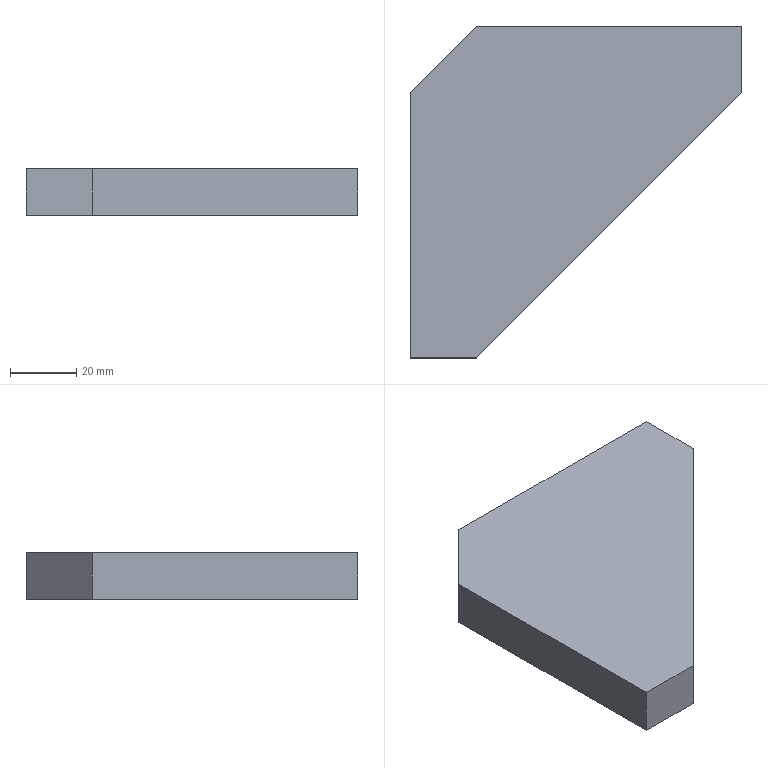Part | SolidWorks | features Extrusion 1 | 1 solid | 8 faces | box 100 x 100 x 14 mm | volume 92400 mm3 | plane 8
STEP:
#1=CARTESIAN_POINT('',(0.,80.,0.));
#2=VERTEX_POINT('',#1);
#3=CARTESIAN_POINT('',(0.,0.,0.));
#4=VERTEX_POINT('',#3);
#5=CARTESIAN_POINT('',(0.,80.,0.));
#6=DIRECTION('',(0.,-1.,0.));
#7=VECTOR('',#6,1000.);
#8=LINE('',#5,#7);
#9=EDGE_CURVE('',#2,#4,#8,.T.);
#10=ORIENTED_EDGE('',*,*,#9,.T.);
#11=CARTESIAN_POINT('',(0.,0.,14.));
#12=VERTEX_POINT('',#11);
#13=CARTESIAN_POINT('',(0.,0.,14.));
#14=DIRECTION('',(0.,0.,-1.));
#15=VECTOR('',#14,1000.);
#16=LINE('',#13,#15);
#17=EDGE_CURVE('',#12,#4,#16,.T.);
#18=ORIENTED_EDGE('',*,*,#17,.F.);
#19=CARTESIAN_POINT('',(0.,80.,14.));
#20=VERTEX_POINT('',#19);
#21=CARTESIAN_POINT('',(0.,80.,14.));
#22=DIRECTION('',(0.,-1.,0.));
#23=VECTOR('',#22,1000.);
#24=LINE('',#21,#23);
#25=EDGE_CURVE('',#20,#12,#24,.T.);
#26=ORIENTED_EDGE('',*,*,#25,.F.);
#27=CARTESIAN_POINT('',(0.,80.,14.));
#28=DIRECTION('',(0.,0.,-1.));
#29=VECTOR('',#28,1000.);
#30=LINE('',#27,#29);
#31=EDGE_CURVE('',#20,#2,#30,.T.);
#32=ORIENTED_EDGE('',*,*,#31,.T.);
#33=EDGE_LOOP('',(#10,#18,#26,#32));
#34=FACE_OUTER_BOUND('',#33,.T.);
#35=CARTESIAN_POINT('',(0.,80.,14.));
#36=DIRECTION('',(1.,0.,0.));
#37=DIRECTION('',(0.,1.,0.));
#38=AXIS2_PLACEMENT_3D('',#35,#36,#37);
#39=PLANE('',#38);
#40=ADVANCED_FACE('',(#34),#39,.F.);
#41=CARTESIAN_POINT('',(20.,0.,0.));
#42=VERTEX_POINT('',#41);
#43=CARTESIAN_POINT('',(0.,0.,0.));
#44=DIRECTION('',(1.,0.,0.));
#45=VECTOR('',#44,1000.);
#46=LINE('',#43,#45);
#47=EDGE_CURVE('',#4,#42,#46,.T.);
#48=ORIENTED_EDGE('',*,*,#47,.T.);
#49=CARTESIAN_POINT('',(20.,0.,14.));
#50=VERTEX_POINT('',#49);
#51=CARTESIAN_POINT('',(20.,0.,14.));
#52=DIRECTION('',(0.,0.,-1.));
#53=VECTOR('',#52,1000.);
#54=LINE('',#51,#53);
#55=EDGE_CURVE('',#50,#42,#54,.T.);
#56=ORIENTED_EDGE('',*,*,#55,.F.);
#57=CARTESIAN_POINT('',(0.,0.,14.));
#58=DIRECTION('',(1.,0.,0.));
#59=VECTOR('',#58,1000.);
#60=LINE('',#57,#59);
#61=EDGE_CURVE('',#12,#50,#60,.T.);
#62=ORIENTED_EDGE('',*,*,#61,.F.);
#63=ORIENTED_EDGE('',*,*,#17,.T.);
#64=EDGE_LOOP('',(#48,#56,#62,#63));
#65=FACE_OUTER_BOUND('',#64,.T.);
#66=CARTESIAN_POINT('',(0.,0.,14.));
#67=DIRECTION('',(0.,1.,0.));
#68=DIRECTION('',(0.,0.,1.));
#69=AXIS2_PLACEMENT_3D('',#66,#67,#68);
#70=PLANE('',#69);
#71=ADVANCED_FACE('',(#65),#70,.F.);
#72=CARTESIAN_POINT('',(100.,80.,0.));
#73=VERTEX_POINT('',#72);
#74=CARTESIAN_POINT('',(20.,0.,0.));
#75=DIRECTION('',(0.7071,0.7071,0.));
#76=VECTOR('',#75,1000.);
#77=LINE('',#74,#76);
#78=EDGE_CURVE('',#42,#73,#77,.T.);
#79=ORIENTED_EDGE('',*,*,#78,.T.);
#80=CARTESIAN_POINT('',(100.,80.,14.));
#81=VERTEX_POINT('',#80);
#82=CARTESIAN_POINT('',(100.,80.,14.));
#83=DIRECTION('',(0.,0.,-1.));
#84=VECTOR('',#83,1000.);
#85=LINE('',#82,#84);
#86=EDGE_CURVE('',#81,#73,#85,.T.);
#87=ORIENTED_EDGE('',*,*,#86,.F.);
#88=CARTESIAN_POINT('',(20.,0.,14.));
#89=DIRECTION('',(0.7071,0.7071,0.));
#90=VECTOR('',#89,1000.);
#91=LINE('',#88,#90);
#92=EDGE_CURVE('',#50,#81,#91,.T.);
#93=ORIENTED_EDGE('',*,*,#92,.F.);
#94=ORIENTED_EDGE('',*,*,#55,.T.);
#95=EDGE_LOOP('',(#79,#87,#93,#94));
#96=FACE_OUTER_BOUND('',#95,.T.);
#97=CARTESIAN_POINT('',(20.,0.,14.));
#98=DIRECTION('',(-0.7071,0.7071,0.));
#99=DIRECTION('',(-0.7071,-0.7071,0.));
#100=AXIS2_PLACEMENT_3D('',#97,#98,#99);
#101=PLANE('',#100);
#102=ADVANCED_FACE('',(#96),#101,.F.);
#103=CARTESIAN_POINT('',(100.,100.,0.));
#104=VERTEX_POINT('',#103);
#105=CARTESIAN_POINT('',(100.,80.,0.));
#106=DIRECTION('',(0.,1.,0.));
#107=VECTOR('',#106,1000.);
#108=LINE('',#105,#107);
#109=EDGE_CURVE('',#73,#104,#108,.T.);
#110=ORIENTED_EDGE('',*,*,#109,.T.);
#111=CARTESIAN_POINT('',(100.,100.,14.));
#112=VERTEX_POINT('',#111);
#113=CARTESIAN_POINT('',(100.,100.,14.));
#114=DIRECTION('',(0.,0.,-1.));
#115=VECTOR('',#114,1000.);
#116=LINE('',#113,#115);
#117=EDGE_CURVE('',#112,#104,#116,.T.);
#118=ORIENTED_EDGE('',*,*,#117,.F.);
#119=CARTESIAN_POINT('',(100.,80.,14.));
#120=DIRECTION('',(0.,1.,0.));
#121=VECTOR('',#120,1000.);
#122=LINE('',#119,#121);
#123=EDGE_CURVE('',#81,#112,#122,.T.);
#124=ORIENTED_EDGE('',*,*,#123,.F.);
#125=ORIENTED_EDGE('',*,*,#86,.T.);
#126=EDGE_LOOP('',(#110,#118,#124,#125));
#127=FACE_OUTER_BOUND('',#126,.T.);
#128=CARTESIAN_POINT('',(100.,80.,14.));
#129=DIRECTION('',(-1.,0.,0.));
#130=DIRECTION('',(0.,0.,1.));
#131=AXIS2_PLACEMENT_3D('',#128,#129,#130);
#132=PLANE('',#131);
#133=ADVANCED_FACE('',(#127),#132,.F.);
#134=CARTESIAN_POINT('',(20.,100.,0.));
#135=VERTEX_POINT('',#134);
#136=CARTESIAN_POINT('',(100.,100.,0.));
#137=DIRECTION('',(-1.,0.,0.));
#138=VECTOR('',#137,1000.);
#139=LINE('',#136,#138);
#140=EDGE_CURVE('',#104,#135,#139,.T.);
#141=ORIENTED_EDGE('',*,*,#140,.T.);
#142=CARTESIAN_POINT('',(20.,100.,14.));
#143=VERTEX_POINT('',#142);
#144=CARTESIAN_POINT('',(20.,100.,14.));
#145=DIRECTION('',(0.,0.,-1.));
#146=VECTOR('',#145,1000.);
#147=LINE('',#144,#146);
#148=EDGE_CURVE('',#143,#135,#147,.T.);
#149=ORIENTED_EDGE('',*,*,#148,.F.);
#150=CARTESIAN_POINT('',(100.,100.,14.));
#151=DIRECTION('',(-1.,0.,0.));
#152=VECTOR('',#151,1000.);
#153=LINE('',#150,#152);
#154=EDGE_CURVE('',#112,#143,#153,.T.);
#155=ORIENTED_EDGE('',*,*,#154,.F.);
#156=ORIENTED_EDGE('',*,*,#117,.T.);
#157=EDGE_LOOP('',(#141,#149,#155,#156));
#158=FACE_OUTER_BOUND('',#157,.T.);
#159=CARTESIAN_POINT('',(100.,100.,14.));
#160=DIRECTION('',(0.,-1.,0.));
#161=DIRECTION('',(1.,0.,0.));
#162=AXIS2_PLACEMENT_3D('',#159,#160,#161);
#163=PLANE('',#162);
#164=ADVANCED_FACE('',(#158),#163,.F.);
#165=CARTESIAN_POINT('',(20.,100.,0.));
#166=DIRECTION('',(-0.7071,-0.7071,0.));
#167=VECTOR('',#166,1000.);
#168=LINE('',#165,#167);
#169=EDGE_CURVE('',#135,#2,#168,.T.);
#170=ORIENTED_EDGE('',*,*,#169,.T.);
#171=ORIENTED_EDGE('',*,*,#31,.F.);
#172=CARTESIAN_POINT('',(20.,100.,14.));
#173=DIRECTION('',(-0.7071,-0.7071,0.));
#174=VECTOR('',#173,1000.);
#175=LINE('',#172,#174);
#176=EDGE_CURVE('',#143,#20,#175,.T.);
#177=ORIENTED_EDGE('',*,*,#176,.F.);
#178=ORIENTED_EDGE('',*,*,#148,.T.);
#179=EDGE_LOOP('',(#170,#171,#177,#178));
#180=FACE_OUTER_BOUND('',#179,.T.);
#181=CARTESIAN_POINT('',(20.,100.,14.));
#182=DIRECTION('',(0.7071,-0.7071,0.));
#183=DIRECTION('',(0.7071,0.7071,0.));
#184=AXIS2_PLACEMENT_3D('',#181,#182,#183);
#185=PLANE('',#184);
#186=ADVANCED_FACE('',(#180),#185,.F.);
#187=ORIENTED_EDGE('',*,*,#25,.T.);
#188=ORIENTED_EDGE('',*,*,#61,.T.);
#189=ORIENTED_EDGE('',*,*,#92,.T.);
#190=ORIENTED_EDGE('',*,*,#123,.T.);
#191=ORIENTED_EDGE('',*,*,#154,.T.);
#192=ORIENTED_EDGE('',*,*,#176,.T.);
#193=EDGE_LOOP('',(#187,#188,#189,#190,#191,#192));
#194=FACE_OUTER_BOUND('',#193,.T.);
#195=CARTESIAN_POINT('',(0.,0.,14.));
#196=DIRECTION('',(0.,0.,1.));
#197=DIRECTION('',(1.,0.,0.));
#198=AXIS2_PLACEMENT_3D('',#195,#196,#197);
#199=PLANE('',#198);
#200=ADVANCED_FACE('',(#194),#199,.T.);
#201=ORIENTED_EDGE('',*,*,#9,.F.);
#202=ORIENTED_EDGE('',*,*,#169,.F.);
#203=ORIENTED_EDGE('',*,*,#140,.F.);
#204=ORIENTED_EDGE('',*,*,#109,.F.);
#205=ORIENTED_EDGE('',*,*,#78,.F.);
#206=ORIENTED_EDGE('',*,*,#47,.F.);
#207=EDGE_LOOP('',(#201,#202,#203,#204,#205,#206));
#208=FACE_OUTER_BOUND('',#207,.T.);
#209=CARTESIAN_POINT('',(0.,0.,0.));
#210=DIRECTION('',(0.,0.,1.));
#211=DIRECTION('',(1.,0.,0.));
#212=AXIS2_PLACEMENT_3D('',#209,#210,#211);
#213=PLANE('',#212);
#214=ADVANCED_FACE('',(#208),#213,.F.);
#215=CLOSED_SHELL('',(#40,#71,#102,#133,#164,#186,#200,#214));
#216=MANIFOLD_SOLID_BREP('',#215);
#217=CARTESIAN_POINT('',(0.,0.,0.));
#218=DIRECTION('',(0.,0.,1.));
#219=DIRECTION('',(1.,0.,0.));
#220=AXIS2_PLACEMENT_3D('',#217,#218,#219);
#221=(LENGTH_UNIT()NAMED_UNIT(*)SI_UNIT(.MILLI.,.METRE.));
#222=UNCERTAINTY_MEASURE_WITH_UNIT(LENGTH_MEASURE(0.00001),#221,'','');
#223=(NAMED_UNIT(*)PLANE_ANGLE_UNIT()SI_UNIT($,.RADIAN.));
#224=(NAMED_UNIT(*)SI_UNIT($,.STERADIAN.)SOLID_ANGLE_UNIT());
#225=(GEOMETRIC_REPRESENTATION_CONTEXT(3)GLOBAL_UNCERTAINTY_ASSIGNED_CONTEXT((#222))GLOBAL_UNIT_ASSIGNED_CONTEXT((#221,#223,#224))REPRESENTATION_CONTEXT('',''));
#226=ADVANCED_BREP_SHAPE_REPRESENTATION('',(#216,#220),#225);